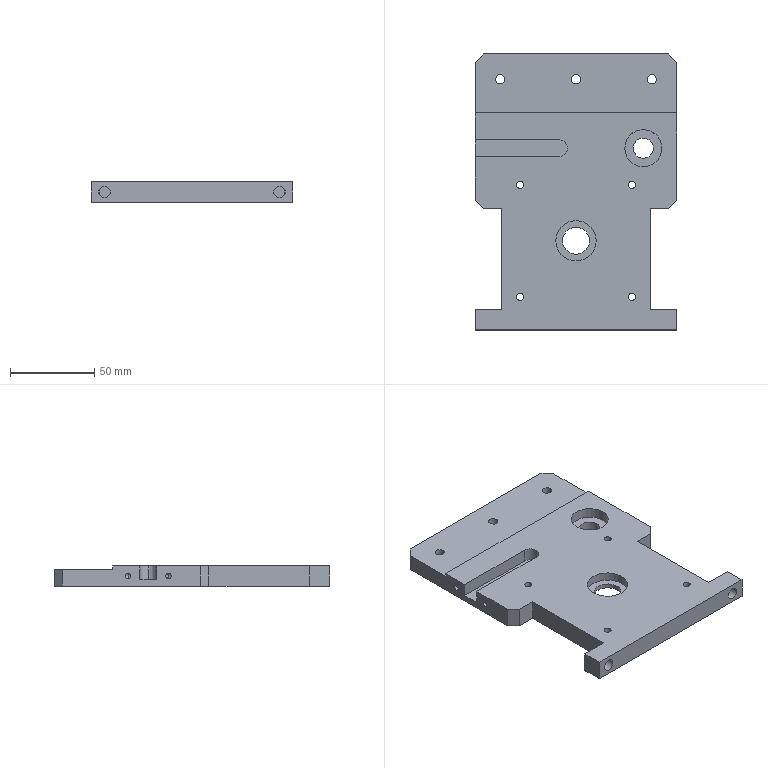Part | STEP file | (PA01.001.LX003) Motor Mounting Plate | 1 solid | 73 faces | box 120 x 164 x 12 mm | volume 186688 mm3 | cylinder 40 | plane 29 | cone 4 | commonest cylinder face diameters 4.2 x8 10 x8 5.5 x6 3.3 x4 7 x4 12 x2